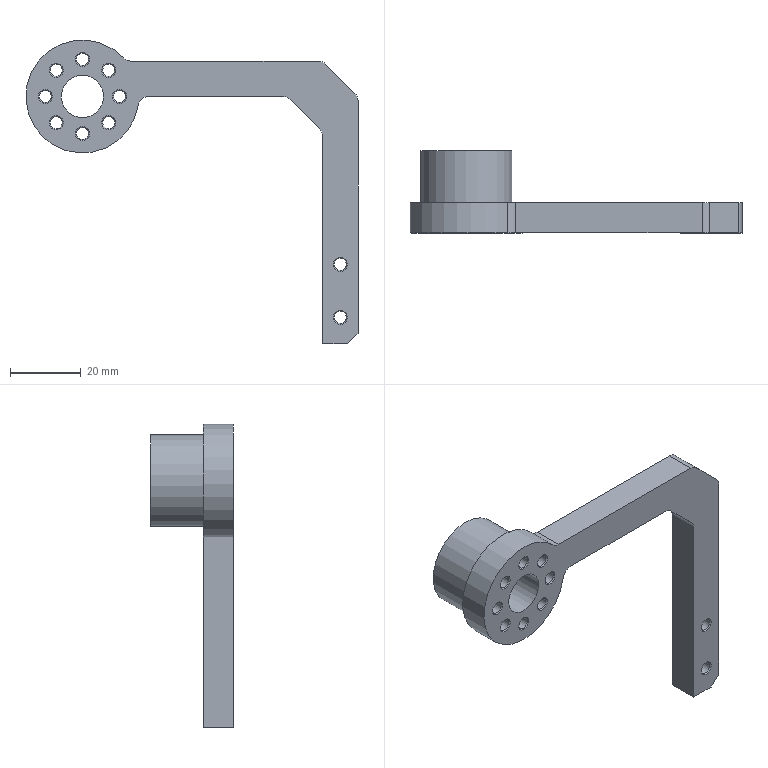Part | NX | features DATUM_CSYS 12, SKETCH 11, SIMPLE HOLE 10, HOLE PACKAGE 9, EXTRACT_FACE 8, Instance Feature 7, CHAMFER 3, BLEND 2, CPROJ 1, EXTRUDE 1, OFFSET_REGION 1, Pattern Feature 1, SWP104 1 | 1 solid | 52 faces | box 93.991 x 23.3 x 85.991 mm | volume 20704 mm3 | cylinder 20 | cone 20 | plane 12 | commonest cylinder face diameters 3.4 x10 6 x6 11.954 x1 25.981 x1 29.983 x1 31.983 x1
STEP:
#1=CARTESIAN_POINT('',(0.,-23.4,-5.977));
#2=VERTEX_POINT('',#1);
#3=CARTESIAN_POINT('',(0.,-23.4,0.));
#4=DIRECTION('',(0.,-1.,0.));
#5=DIRECTION('',(0.,0.,-1.));
#6=AXIS2_PLACEMENT_3D('',#3,#4,#5);
#7=CIRCLE('',#6,5.977);
#8=EDGE_CURVE('',#2,#2,#7,.T.);
#9=ORIENTED_EDGE('',*,*,#8,.T.);
#10=EDGE_LOOP('',(#9));
#11=FACE_BOUND('',#10,.T.);
#12=CARTESIAN_POINT('',(0.,-0.1,-5.977));
#13=VERTEX_POINT('',#12);
#14=CARTESIAN_POINT('',(0.,-0.1,0.));
#15=DIRECTION('',(0.,-1.,0.));
#16=DIRECTION('',(0.,0.,-1.));
#17=AXIS2_PLACEMENT_3D('',#14,#15,#16);
#18=CIRCLE('',#17,5.977);
#19=EDGE_CURVE('',#13,#13,#18,.T.);
#20=ORIENTED_EDGE('',*,*,#19,.F.);
#21=EDGE_LOOP('',(#20));
#22=FACE_BOUND('',#21,.T.);
#23=CARTESIAN_POINT('',(0.,0.,0.));
#24=DIRECTION('',(0.,-1.,0.));
#25=DIRECTION('',(0.,0.,-1.));
#26=AXIS2_PLACEMENT_3D('',#23,#24,#25);
#27=CYLINDRICAL_SURFACE('',#26,5.977);
#28=ADVANCED_FACE('',(#11,#22),#27,.F.);
#29=CARTESIAN_POINT('',(73.,-23.4,-64.5));
#30=VERTEX_POINT('',#29);
#31=CARTESIAN_POINT('',(73.,-23.4,-62.5));
#32=DIRECTION('',(0.,-1.,0.));
#33=DIRECTION('',(0.,0.,-1.));
#34=AXIS2_PLACEMENT_3D('',#31,#32,#33);
#35=CIRCLE('',#34,2.);
#36=EDGE_CURVE('',#30,#30,#35,.F.);
#37=ORIENTED_EDGE('',*,*,#36,.T.);
#38=EDGE_LOOP('',(#37));
#39=FACE_BOUND('',#38,.T.);
#40=CARTESIAN_POINT('',(73.,-23.4,-49.5));
#41=VERTEX_POINT('',#40);
#42=CARTESIAN_POINT('',(73.,-23.4,-47.5));
#43=DIRECTION('',(0.,-1.,0.));
#44=DIRECTION('',(0.,0.,-1.));
#45=AXIS2_PLACEMENT_3D('',#42,#43,#44);
#46=CIRCLE('',#45,2.);
#47=EDGE_CURVE('',#41,#41,#46,.F.);
#48=ORIENTED_EDGE('',*,*,#47,.T.);
#49=EDGE_LOOP('',(#48));
#50=FACE_BOUND('',#49,.T.);
#51=CARTESIAN_POINT('',(7.425,-23.4,5.425));
#52=VERTEX_POINT('',#51);
#53=CARTESIAN_POINT('',(7.425,-23.4,7.425));
#54=DIRECTION('',(0.,-1.,0.));
#55=DIRECTION('',(0.,0.,-1.));
#56=AXIS2_PLACEMENT_3D('',#53,#54,#55);
#57=CIRCLE('',#56,2.);
#58=EDGE_CURVE('',#52,#52,#57,.F.);
#59=ORIENTED_EDGE('',*,*,#58,.T.);
#60=EDGE_LOOP('',(#59));
#61=FACE_BOUND('',#60,.T.);
#62=CARTESIAN_POINT('',(10.5,-23.4,-2.));
#63=VERTEX_POINT('',#62);
#64=CARTESIAN_POINT('',(10.5,-23.4,0.));
#65=DIRECTION('',(0.,-1.,0.));
#66=DIRECTION('',(0.,0.,-1.));
#67=AXIS2_PLACEMENT_3D('',#64,#65,#66);
#68=CIRCLE('',#67,2.);
#69=EDGE_CURVE('',#63,#63,#68,.F.);
#70=ORIENTED_EDGE('',*,*,#69,.T.);
#71=EDGE_LOOP('',(#70));
#72=FACE_BOUND('',#71,.T.);
#73=CARTESIAN_POINT('',(7.425,-23.4,-9.425));
#74=VERTEX_POINT('',#73);
#75=CARTESIAN_POINT('',(7.425,-23.4,-7.425));
#76=DIRECTION('',(0.,-1.,0.));
#77=DIRECTION('',(0.,0.,-1.));
#78=AXIS2_PLACEMENT_3D('',#75,#76,#77);
#79=CIRCLE('',#78,2.);
#80=EDGE_CURVE('',#74,#74,#79,.F.);
#81=ORIENTED_EDGE('',*,*,#80,.T.);
#82=EDGE_LOOP('',(#81));
#83=FACE_BOUND('',#82,.T.);
#84=CARTESIAN_POINT('',(0.,-23.4,-12.5));
#85=VERTEX_POINT('',#84);
#86=CARTESIAN_POINT('',(0.,-23.4,-10.5));
#87=DIRECTION('',(0.,-1.,0.));
#88=DIRECTION('',(0.,0.,-1.));
#89=AXIS2_PLACEMENT_3D('',#86,#87,#88);
#90=CIRCLE('',#89,2.);
#91=EDGE_CURVE('',#85,#85,#90,.F.);
#92=ORIENTED_EDGE('',*,*,#91,.T.);
#93=EDGE_LOOP('',(#92));
#94=FACE_BOUND('',#93,.T.);
#95=CARTESIAN_POINT('',(-7.425,-23.4,-9.425));
#96=VERTEX_POINT('',#95);
#97=CARTESIAN_POINT('',(-7.425,-23.4,-7.425));
#98=DIRECTION('',(0.,-1.,0.));
#99=DIRECTION('',(0.,0.,-1.));
#100=AXIS2_PLACEMENT_3D('',#97,#98,#99);
#101=CIRCLE('',#100,2.);
#102=EDGE_CURVE('',#96,#96,#101,.F.);
#103=ORIENTED_EDGE('',*,*,#102,.T.);
#104=EDGE_LOOP('',(#103));
#105=FACE_BOUND('',#104,.T.);
#106=CARTESIAN_POINT('',(-10.5,-23.4,-2.));
#107=VERTEX_POINT('',#106);
#108=CARTESIAN_POINT('',(-10.5,-23.4,0.));
#109=DIRECTION('',(0.,-1.,0.));
#110=DIRECTION('',(0.,0.,-1.));
#111=AXIS2_PLACEMENT_3D('',#108,#109,#110);
#112=CIRCLE('',#111,2.);
#113=EDGE_CURVE('',#107,#107,#112,.F.);
#114=ORIENTED_EDGE('',*,*,#113,.T.);
#115=EDGE_LOOP('',(#114));
#116=FACE_BOUND('',#115,.T.);
#117=CARTESIAN_POINT('',(-7.425,-23.4,5.425));
#118=VERTEX_POINT('',#117);
#119=CARTESIAN_POINT('',(-7.425,-23.4,7.425));
#120=DIRECTION('',(0.,-1.,0.));
#121=DIRECTION('',(0.,0.,-1.));
#122=AXIS2_PLACEMENT_3D('',#119,#120,#121);
#123=CIRCLE('',#122,2.);
#124=EDGE_CURVE('',#118,#118,#123,.F.);
#125=ORIENTED_EDGE('',*,*,#124,.T.);
#126=EDGE_LOOP('',(#125));
#127=FACE_BOUND('',#126,.T.);
#128=CARTESIAN_POINT('',(0.,-23.4,8.5));
#129=VERTEX_POINT('',#128);
#130=CARTESIAN_POINT('',(0.,-23.4,10.5));
#131=DIRECTION('',(0.,-1.,0.));
#132=DIRECTION('',(0.,0.,-1.));
#133=AXIS2_PLACEMENT_3D('',#130,#131,#132);
#134=CIRCLE('',#133,2.);
#135=EDGE_CURVE('',#129,#129,#134,.F.);
#136=ORIENTED_EDGE('',*,*,#135,.T.);
#137=EDGE_LOOP('',(#136));
#138=FACE_BOUND('',#137,.T.);
#139=CARTESIAN_POINT('',(68.,-23.4,-70.));
#140=VERTEX_POINT('',#139);
#141=CARTESIAN_POINT('',(75.,-23.4,-70.));
#142=VERTEX_POINT('',#141);
#143=CARTESIAN_POINT('',(68.,-23.4,-70.));
#144=DIRECTION('',(1.,0.,0.));
#145=VECTOR('',#144,1000.);
#146=LINE('',#143,#145);
#147=EDGE_CURVE('',#140,#142,#146,.T.);
#148=ORIENTED_EDGE('',*,*,#147,.T.);
#149=CARTESIAN_POINT('',(78.,-23.4,-67.));
#150=VERTEX_POINT('',#149);
#151=CARTESIAN_POINT('',(75.489,-23.4,-69.511));
#152=DIRECTION('',(-0.7071,0.,-0.7071));
#153=VECTOR('',#152,1000.);
#154=LINE('',#151,#153);
#155=EDGE_CURVE('',#142,#150,#154,.F.);
#156=ORIENTED_EDGE('',*,*,#155,.T.);
#157=CARTESIAN_POINT('',(78.,-23.4,-1.243));
#158=VERTEX_POINT('',#157);
#159=CARTESIAN_POINT('',(78.,-23.4,0.));
#160=DIRECTION('',(0.,0.,1.));
#161=VECTOR('',#160,1000.);
#162=LINE('',#159,#161);
#163=EDGE_CURVE('',#150,#158,#162,.T.);
#164=ORIENTED_EDGE('',*,*,#163,.T.);
#165=CARTESIAN_POINT('',(77.121,-23.4,0.8787));
#166=VERTEX_POINT('',#165);
#167=CARTESIAN_POINT('',(75.,-23.4,-1.243));
#168=DIRECTION('',(0.,-1.,0.));
#169=DIRECTION('',(0.,0.,-1.));
#170=AXIS2_PLACEMENT_3D('',#167,#168,#169);
#171=CIRCLE('',#170,3.);
#172=EDGE_CURVE('',#158,#166,#171,.T.);
#173=ORIENTED_EDGE('',*,*,#172,.T.);
#174=CARTESIAN_POINT('',(68.879,-23.4,9.121));
#175=VERTEX_POINT('',#174);
#176=CARTESIAN_POINT('',(41.989,-23.4,36.011));
#177=DIRECTION('',(0.7071,0.,-0.7071));
#178=VECTOR('',#177,1000.);
#179=LINE('',#176,#178);
#180=EDGE_CURVE('',#166,#175,#179,.F.);
#181=ORIENTED_EDGE('',*,*,#180,.T.);
#182=CARTESIAN_POINT('',(66.757,-23.4,10.));
#183=VERTEX_POINT('',#182);
#184=CARTESIAN_POINT('',(66.757,-23.4,7.));
#185=DIRECTION('',(0.,-1.,0.));
#186=DIRECTION('',(0.,0.,-1.));
#187=AXIS2_PLACEMENT_3D('',#184,#185,#186);
#188=CIRCLE('',#187,3.);
#189=EDGE_CURVE('',#175,#183,#188,.T.);
#190=ORIENTED_EDGE('',*,*,#189,.T.);
#191=CARTESIAN_POINT('',(13.845,-23.4,10.));
#192=VERTEX_POINT('',#191);
#193=CARTESIAN_POINT('',(68.,-23.4,10.));
#194=DIRECTION('',(-1.,0.,0.));
#195=VECTOR('',#194,1000.);
#196=LINE('',#193,#195);
#197=EDGE_CURVE('',#183,#192,#196,.T.);
#198=ORIENTED_EDGE('',*,*,#197,.T.);
#199=CARTESIAN_POINT('',(11.658,-23.4,10.946));
#200=VERTEX_POINT('',#199);
#201=CARTESIAN_POINT('',(13.845,-23.4,13.));
#202=DIRECTION('',(0.,-1.,0.));
#203=DIRECTION('',(0.,0.,-1.));
#204=AXIS2_PLACEMENT_3D('',#201,#202,#203);
#205=CIRCLE('',#204,3.);
#206=EDGE_CURVE('',#192,#200,#205,.F.);
#207=ORIENTED_EDGE('',*,*,#206,.T.);
#208=CARTESIAN_POINT('',(15.791,-23.4,-2.526));
#209=VERTEX_POINT('',#208);
#210=CARTESIAN_POINT('',(0.,-23.4,0.));
#211=DIRECTION('',(0.,-1.,0.));
#212=DIRECTION('',(0.,0.,-1.));
#213=AXIS2_PLACEMENT_3D('',#210,#211,#212);
#214=CIRCLE('',#213,15.991);
#215=EDGE_CURVE('',#200,#209,#214,.T.);
#216=ORIENTED_EDGE('',*,*,#215,.T.);
#217=CARTESIAN_POINT('',(18.753,-23.4,0.));
#218=VERTEX_POINT('',#217);
#219=CARTESIAN_POINT('',(18.753,-23.4,-3.));
#220=DIRECTION('',(0.,-1.,0.));
#221=DIRECTION('',(0.,0.,-1.));
#222=AXIS2_PLACEMENT_3D('',#219,#220,#221);
#223=CIRCLE('',#222,3.);
#224=EDGE_CURVE('',#209,#218,#223,.F.);
#225=ORIENTED_EDGE('',*,*,#224,.T.);
#226=CARTESIAN_POINT('',(56.757,-23.4,0.));
#227=VERTEX_POINT('',#226);
#228=CARTESIAN_POINT('',(15.991,-23.4,0.));
#229=DIRECTION('',(1.,0.,0.));
#230=VECTOR('',#229,1000.);
#231=LINE('',#228,#230);
#232=EDGE_CURVE('',#218,#227,#231,.T.);
#233=ORIENTED_EDGE('',*,*,#232,.T.);
#234=CARTESIAN_POINT('',(58.879,-23.4,-0.8787));
#235=VERTEX_POINT('',#234);
#236=CARTESIAN_POINT('',(56.757,-23.4,-3.));
#237=DIRECTION('',(0.,-1.,0.));
#238=DIRECTION('',(0.,0.,-1.));
#239=AXIS2_PLACEMENT_3D('',#236,#237,#238);
#240=CIRCLE('',#239,3.);
#241=EDGE_CURVE('',#227,#235,#240,.F.);
#242=ORIENTED_EDGE('',*,*,#241,.T.);
#243=CARTESIAN_POINT('',(67.121,-23.4,-9.121));
#244=VERTEX_POINT('',#243);
#245=CARTESIAN_POINT('',(58.,-23.4,0.));
#246=DIRECTION('',(-0.7071,0.,0.7071));
#247=VECTOR('',#246,1000.);
#248=LINE('',#245,#247);
#249=EDGE_CURVE('',#235,#244,#248,.F.);
#250=ORIENTED_EDGE('',*,*,#249,.T.);
#251=CARTESIAN_POINT('',(68.,-23.4,-11.243));
#252=VERTEX_POINT('',#251);
#253=CARTESIAN_POINT('',(65.,-23.4,-11.243));
#254=DIRECTION('',(0.,-1.,0.));
#255=DIRECTION('',(0.,0.,-1.));
#256=AXIS2_PLACEMENT_3D('',#253,#254,#255);
#257=CIRCLE('',#256,3.);
#258=EDGE_CURVE('',#244,#252,#257,.F.);
#259=ORIENTED_EDGE('',*,*,#258,.T.);
#260=CARTESIAN_POINT('',(68.,-23.4,0.));
#261=DIRECTION('',(0.,0.,-1.));
#262=VECTOR('',#261,1000.);
#263=LINE('',#260,#262);
#264=EDGE_CURVE('',#252,#140,#263,.T.);
#265=ORIENTED_EDGE('',*,*,#264,.T.);
#266=EDGE_LOOP('',(#148,#156,#164,#173,#181,#190,#198,#207,#216,#225,#233,#242,#250,#259,#265));
#267=FACE_BOUND('',#266,.T.);
#268=ORIENTED_EDGE('',*,*,#8,.F.);
#269=EDGE_LOOP('',(#268));
#270=FACE_BOUND('',#269,.T.);
#271=CARTESIAN_POINT('',(5.977,-23.4,0.));
#272=DIRECTION('',(0.,-1.,0.));
#273=DIRECTION('',(0.,0.,-1.));
#274=AXIS2_PLACEMENT_3D('',#271,#272,#273);
#275=PLANE('',#274);
#276=ADVANCED_FACE('',(#39,#50,#61,#72,#83,#94,#105,#116,#127,#138,#267,#270),#275,.T.);
#277=CARTESIAN_POINT('',(11.658,-14.9,10.946));
#278=VERTEX_POINT('',#277);
#279=CARTESIAN_POINT('',(15.791,-14.9,-2.526));
#280=VERTEX_POINT('',#279);
#281=CARTESIAN_POINT('',(0.,-14.9,0.));
#282=DIRECTION('',(0.,-1.,0.));
#283=DIRECTION('',(0.,0.,-1.));
#284=AXIS2_PLACEMENT_3D('',#281,#282,#283);
#285=CIRCLE('',#284,15.991);
#286=EDGE_CURVE('',#278,#280,#285,.T.);
#287=ORIENTED_EDGE('',*,*,#286,.T.);
#288=CARTESIAN_POINT('',(15.791,0.,-2.526));
#289=DIRECTION('',(0.,-1.,0.));
#290=VECTOR('',#289,1000.);
#291=LINE('',#288,#290);
#292=EDGE_CURVE('',#280,#209,#291,.T.);
#293=ORIENTED_EDGE('',*,*,#292,.T.);
#294=ORIENTED_EDGE('',*,*,#215,.F.);
#295=CARTESIAN_POINT('',(11.658,0.,10.946));
#296=DIRECTION('',(0.,-1.,0.));
#297=VECTOR('',#296,1000.);
#298=LINE('',#295,#297);
#299=EDGE_CURVE('',#200,#278,#298,.F.);
#300=ORIENTED_EDGE('',*,*,#299,.T.);
#301=EDGE_LOOP('',(#287,#293,#294,#300));
#302=FACE_BOUND('',#301,.T.);
#303=CARTESIAN_POINT('',(0.,0.,0.));
#304=DIRECTION('',(0.,-1.,0.));
#305=DIRECTION('',(0.,0.,-1.));
#306=AXIS2_PLACEMENT_3D('',#303,#304,#305);
#307=CYLINDRICAL_SURFACE('',#306,15.991);
#308=ADVANCED_FACE('',(#302),#307,.T.);
#309=CARTESIAN_POINT('',(73.,-14.9,-60.5));
#310=VERTEX_POINT('',#309);
#311=CARTESIAN_POINT('',(73.,-14.9,-62.5));
#312=DIRECTION('',(0.,1.,0.));
#313=DIRECTION('',(0.,0.,1.));
#314=AXIS2_PLACEMENT_3D('',#311,#312,#313);
#315=CIRCLE('',#314,2.);
#316=EDGE_CURVE('',#310,#310,#315,.F.);
#317=ORIENTED_EDGE('',*,*,#316,.T.);
#318=EDGE_LOOP('',(#317));
#319=FACE_BOUND('',#318,.T.);
#320=CARTESIAN_POINT('',(73.,-14.9,-45.5));
#321=VERTEX_POINT('',#320);
#322=CARTESIAN_POINT('',(73.,-14.9,-47.5));
#323=DIRECTION('',(0.,1.,0.));
#324=DIRECTION('',(0.,0.,1.));
#325=AXIS2_PLACEMENT_3D('',#322,#323,#324);
#326=CIRCLE('',#325,2.);
#327=EDGE_CURVE('',#321,#321,#326,.F.);
#328=ORIENTED_EDGE('',*,*,#327,.T.);
#329=EDGE_LOOP('',(#328));
#330=FACE_BOUND('',#329,.T.);
#331=CARTESIAN_POINT('',(0.,-14.9,-14.991));
#332=VERTEX_POINT('',#331);
#333=CARTESIAN_POINT('',(0.,-14.9,0.));
#334=DIRECTION('',(0.,-1.,0.));
#335=DIRECTION('',(0.,0.,-1.));
#336=AXIS2_PLACEMENT_3D('',#333,#334,#335);
#337=CIRCLE('',#336,14.991);
#338=EDGE_CURVE('',#332,#332,#337,.T.);
#339=ORIENTED_EDGE('',*,*,#338,.T.);
#340=EDGE_LOOP('',(#339));
#341=FACE_BOUND('',#340,.T.);
#342=CARTESIAN_POINT('',(78.,-14.9,-67.));
#343=VERTEX_POINT('',#342);
#344=CARTESIAN_POINT('',(78.,-14.9,-1.243));
#345=VERTEX_POINT('',#344);
#346=CARTESIAN_POINT('',(78.,-14.9,-70.));
#347=DIRECTION('',(0.,0.,1.));
#348=VECTOR('',#347,1000.);
#349=LINE('',#346,#348);
#350=EDGE_CURVE('',#343,#345,#349,.T.);
#351=ORIENTED_EDGE('',*,*,#350,.F.);
#352=CARTESIAN_POINT('',(75.,-14.9,-70.));
#353=VERTEX_POINT('',#352);
#354=CARTESIAN_POINT('',(80.496,-14.9,-64.504));
#355=DIRECTION('',(0.7071,0.,0.7071));
#356=VECTOR('',#355,1000.);
#357=LINE('',#354,#356);
#358=EDGE_CURVE('',#343,#353,#357,.F.);
#359=ORIENTED_EDGE('',*,*,#358,.T.);
#360=CARTESIAN_POINT('',(68.,-14.9,-70.));
#361=VERTEX_POINT('',#360);
#362=CARTESIAN_POINT('',(68.,-14.9,-70.));
#363=DIRECTION('',(1.,0.,0.));
#364=VECTOR('',#363,1000.);
#365=LINE('',#362,#364);
#366=EDGE_CURVE('',#361,#353,#365,.T.);
#367=ORIENTED_EDGE('',*,*,#366,.F.);
#368=CARTESIAN_POINT('',(68.,-14.9,-11.243));
#369=VERTEX_POINT('',#368);
#370=CARTESIAN_POINT('',(68.,-14.9,0.));
#371=DIRECTION('',(0.,0.,-1.));
#372=VECTOR('',#371,1000.);
#373=LINE('',#370,#372);
#374=EDGE_CURVE('',#369,#361,#373,.T.);
#375=ORIENTED_EDGE('',*,*,#374,.F.);
#376=CARTESIAN_POINT('',(67.121,-14.9,-9.121));
#377=VERTEX_POINT('',#376);
#378=CARTESIAN_POINT('',(65.,-14.9,-11.243));
#379=DIRECTION('',(0.,1.,0.));
#380=DIRECTION('',(0.,0.,1.));
#381=AXIS2_PLACEMENT_3D('',#378,#379,#380);
#382=CIRCLE('',#381,3.);
#383=EDGE_CURVE('',#369,#377,#382,.F.);
#384=ORIENTED_EDGE('',*,*,#383,.T.);
#385=CARTESIAN_POINT('',(58.879,-14.9,-0.8787));
#386=VERTEX_POINT('',#385);
#387=CARTESIAN_POINT('',(58.,-14.9,0.));
#388=DIRECTION('',(0.7071,0.,-0.7071));
#389=VECTOR('',#388,1000.);
#390=LINE('',#387,#389);
#391=EDGE_CURVE('',#377,#386,#390,.F.);
#392=ORIENTED_EDGE('',*,*,#391,.T.);
#393=CARTESIAN_POINT('',(56.757,-14.9,0.));
#394=VERTEX_POINT('',#393);
#395=CARTESIAN_POINT('',(56.757,-14.9,-3.));
#396=DIRECTION('',(0.,1.,0.));
#397=DIRECTION('',(0.,0.,1.));
#398=AXIS2_PLACEMENT_3D('',#395,#396,#397);
#399=CIRCLE('',#398,3.);
#400=EDGE_CURVE('',#386,#394,#399,.F.);
#401=ORIENTED_EDGE('',*,*,#400,.T.);
#402=CARTESIAN_POINT('',(18.753,-14.9,0.));
#403=VERTEX_POINT('',#402);
#404=CARTESIAN_POINT('',(15.991,-14.9,0.));
#405=DIRECTION('',(1.,0.,0.));
#406=VECTOR('',#405,1000.);
#407=LINE('',#404,#406);
#408=EDGE_CURVE('',#403,#394,#407,.T.);
#409=ORIENTED_EDGE('',*,*,#408,.F.);
#410=CARTESIAN_POINT('',(18.753,-14.9,-3.));
#411=DIRECTION('',(0.,1.,0.));
#412=DIRECTION('',(0.,0.,1.));
#413=AXIS2_PLACEMENT_3D('',#410,#411,#412);
#414=CIRCLE('',#413,3.);
#415=EDGE_CURVE('',#403,#280,#414,.F.);
#416=ORIENTED_EDGE('',*,*,#415,.T.);
#417=ORIENTED_EDGE('',*,*,#286,.F.);
#418=CARTESIAN_POINT('',(13.845,-14.9,10.));
#419=VERTEX_POINT('',#418);
#420=CARTESIAN_POINT('',(13.845,-14.9,13.));
#421=DIRECTION('',(0.,1.,0.));
#422=DIRECTION('',(0.,0.,1.));
#423=AXIS2_PLACEMENT_3D('',#420,#421,#422);
#424=CIRCLE('',#423,3.);
#425=EDGE_CURVE('',#278,#419,#424,.F.);
#426=ORIENTED_EDGE('',*,*,#425,.T.);
#427=CARTESIAN_POINT('',(66.757,-14.9,10.));
#428=VERTEX_POINT('',#427);
#429=CARTESIAN_POINT('',(78.,-14.9,10.));
#430=DIRECTION('',(-1.,0.,0.));
#431=VECTOR('',#430,1000.);
#432=LINE('',#429,#431);
#433=EDGE_CURVE('',#428,#419,#432,.T.);
#434=ORIENTED_EDGE('',*,*,#433,.F.);
#435=CARTESIAN_POINT('',(68.879,-14.9,9.121));
#436=VERTEX_POINT('',#435);
#437=CARTESIAN_POINT('',(66.757,-14.9,7.));
#438=DIRECTION('',(0.,1.,0.));
#439=DIRECTION('',(0.,0.,1.));
#440=AXIS2_PLACEMENT_3D('',#437,#438,#439);
#441=CIRCLE('',#440,3.);
#442=EDGE_CURVE('',#428,#436,#441,.T.);
#443=ORIENTED_EDGE('',*,*,#442,.T.);
#444=CARTESIAN_POINT('',(77.121,-14.9,0.8787));
#445=VERTEX_POINT('',#444);
#446=CARTESIAN_POINT('',(46.996,-14.9,31.004));
#447=DIRECTION('',(-0.7071,0.,0.7071));
#448=VECTOR('',#447,1000.);
#449=LINE('',#446,#448);
#450=EDGE_CURVE('',#436,#445,#449,.F.);
#451=ORIENTED_EDGE('',*,*,#450,.T.);
#452=CARTESIAN_POINT('',(75.,-14.9,-1.243));
#453=DIRECTION('',(0.,1.,0.));
#454=DIRECTION('',(0.,0.,1.));
#455=AXIS2_PLACEMENT_3D('',#452,#453,#454);
#456=CIRCLE('',#455,3.);
#457=EDGE_CURVE('',#445,#345,#456,.T.);
#458=ORIENTED_EDGE('',*,*,#457,.T.);
#459=EDGE_LOOP('',(#351,#359,#367,#375,#384,#392,#401,#409,#416,#417,#426,#434,#443,#451,#458));
#460=FACE_BOUND('',#459,.T.);
#461=CARTESIAN_POINT('',(15.991,-14.9,0.));
#462=DIRECTION('',(0.,1.,0.));
#463=DIRECTION('',(0.,0.,1.));
#464=AXIS2_PLACEMENT_3D('',#461,#462,#463);
#465=PLANE('',#464);
#466=ADVANCED_FACE('',(#319,#330,#341,#460),#465,.T.);
#467=CARTESIAN_POINT('',(0.,-19.4,14.991));
#468=VERTEX_POINT('',#467);
#469=CARTESIAN_POINT('',(0.,-19.4,0.));
#470=DIRECTION('',(0.,1.,0.));
#471=DIRECTION('',(0.,0.,1.));
#472=AXIS2_PLACEMENT_3D('',#469,#470,#471);
#473=CIRCLE('',#472,14.991);
#474=EDGE_CURVE('',#468,#468,#473,.F.);
#475=ORIENTED_EDGE('',*,*,#474,.T.);
#476=EDGE_LOOP('',(#475));
#477=FACE_BOUND('',#476,.T.);
#478=ORIENTED_EDGE('',*,*,#338,.F.);
#479=EDGE_LOOP('',(#478));
#480=FACE_BOUND('',#479,.T.);
#481=CARTESIAN_POINT('',(0.,0.,0.));
#482=DIRECTION('',(0.,-1.,0.));
#483=DIRECTION('',(0.,0.,-1.));
#484=AXIS2_PLACEMENT_3D('',#481,#482,#483);
#485=CYLINDRICAL_SURFACE('',#484,14.991);
#486=ADVANCED_FACE('',(#477,#480),#485,.F.);
#487=CARTESIAN_POINT('',(0.,-19.4,12.991));
#488=VERTEX_POINT('',#487);
#489=CARTESIAN_POINT('',(0.,-19.4,0.));
#490=DIRECTION('',(0.,1.,0.));
#491=DIRECTION('',(0.,0.,1.));
#492=AXIS2_PLACEMENT_3D('',#489,#490,#491);
#493=CIRCLE('',#492,12.991);
#494=EDGE_CURVE('',#488,#488,#493,.F.);
#495=ORIENTED_EDGE('',*,*,#494,.T.);
#496=EDGE_LOOP('',(#495));
#497=FACE_BOUND('',#496,.T.);
#498=ORIENTED_EDGE('',*,*,#474,.F.);
#499=EDGE_LOOP('',(#498));
#500=FACE_BOUND('',#499,.T.);
#501=CARTESIAN_POINT('',(14.991,-19.4,0.));
#502=DIRECTION('',(0.,1.,0.));
#503=DIRECTION('',(0.,0.,1.));
#504=AXIS2_PLACEMENT_3D('',#501,#502,#503);
#505=PLANE('',#504);
#506=ADVANCED_FACE('',(#497,#500),#505,.T.);
#507=CARTESIAN_POINT('',(0.,-0.1,-12.991));
#508=VERTEX_POINT('',#507);
#509=CARTESIAN_POINT('',(0.,-0.1,0.));
#510=DIRECTION('',(0.,-1.,0.));
#511=DIRECTION('',(0.,0.,-1.));
#512=AXIS2_PLACEMENT_3D('',#509,#510,#511);
#513=CIRCLE('',#512,12.991);
#514=EDGE_CURVE('',#508,#508,#513,.T.);
#515=ORIENTED_EDGE('',*,*,#514,.T.);
#516=EDGE_LOOP('',(#515));
#517=FACE_BOUND('',#516,.T.);
#518=ORIENTED_EDGE('',*,*,#494,.F.);
#519=EDGE_LOOP('',(#518));
#520=FACE_BOUND('',#519,.T.);
#521=CARTESIAN_POINT('',(0.,0.,0.));
#522=DIRECTION('',(0.,-1.,0.));
#523=DIRECTION('',(0.,0.,-1.));
#524=AXIS2_PLACEMENT_3D('',#521,#522,#523);
#525=CYLINDRICAL_SURFACE('',#524,12.991);
#526=ADVANCED_FACE('',(#517,#520),#525,.T.);
#527=CARTESIAN_POINT('',(7.425,-0.1,9.425));
#528=VERTEX_POINT('',#527);
#529=CARTESIAN_POINT('',(7.425,-0.1,7.425));
#530=DIRECTION('',(0.,1.,0.));
#531=DIRECTION('',(0.,0.,1.));
#532=AXIS2_PLACEMENT_3D('',#529,#530,#531);
#533=CIRCLE('',#532,2.);
#534=EDGE_CURVE('',#528,#528,#533,.F.);
#535=ORIENTED_EDGE('',*,*,#534,.T.);
#536=EDGE_LOOP('',(#535));
#537=FACE_BOUND('',#536,.T.);
#538=CARTESIAN_POINT('',(10.5,-0.1,2.));
#539=VERTEX_POINT('',#538);
#540=CARTESIAN_POINT('',(10.5,-0.1,0.));
#541=DIRECTION('',(0.,1.,0.));
#542=DIRECTION('',(0.,0.,1.));
#543=AXIS2_PLACEMENT_3D('',#540,#541,#542);
#544=CIRCLE('',#543,2.);
#545=EDGE_CURVE('',#539,#539,#544,.F.);
#546=ORIENTED_EDGE('',*,*,#545,.T.);
#547=EDGE_LOOP('',(#546));
#548=FACE_BOUND('',#547,.T.);
#549=CARTESIAN_POINT('',(7.425,-0.1,-5.425));
#550=VERTEX_POINT('',#549);
#551=CARTESIAN_POINT('',(7.425,-0.1,-7.425));
#552=DIRECTION('',(0.,1.,0.));
#553=DIRECTION('',(0.,0.,1.));
#554=AXIS2_PLACEMENT_3D('',#551,#552,#553);
#555=CIRCLE('',#554,2.);
#556=EDGE_CURVE('',#550,#550,#555,.F.);
#557=ORIENTED_EDGE('',*,*,#556,.T.);
#558=EDGE_LOOP('',(#557));
#559=FACE_BOUND('',#558,.T.);
#560=CARTESIAN_POINT('',(0.,-0.1,-8.5));
#561=VERTEX_POINT('',#560);
#562=CARTESIAN_POINT('',(0.,-0.1,-10.5));
#563=DIRECTION('',(0.,1.,0.));
#564=DIRECTION('',(0.,0.,1.));
#565=AXIS2_PLACEMENT_3D('',#562,#563,#564);
#566=CIRCLE('',#565,2.);
#567=EDGE_CURVE('',#561,#561,#566,.F.);
#568=ORIENTED_EDGE('',*,*,#567,.T.);
#569=EDGE_LOOP('',(#568));
#570=FACE_BOUND('',#569,.T.);
#571=CARTESIAN_POINT('',(-7.425,-0.1,-5.425));
#572=VERTEX_POINT('',#571);
#573=CARTESIAN_POINT('',(-7.425,-0.1,-7.425));
#574=DIRECTION('',(0.,1.,0.));
#575=DIRECTION('',(0.,0.,1.));
#576=AXIS2_PLACEMENT_3D('',#573,#574,#575);
#577=CIRCLE('',#576,2.);
#578=EDGE_CURVE('',#572,#572,#577,.F.);
#579=ORIENTED_EDGE('',*,*,#578,.T.);
#580=EDGE_LOOP('',(#579));
#581=FACE_BOUND('',#580,.T.);
#582=CARTESIAN_POINT('',(-10.5,-0.1,2.));
#583=VERTEX_POINT('',#582);
#584=CARTESIAN_POINT('',(-10.5,-0.1,0.));
#585=DIRECTION('',(0.,1.,0.));
#586=DIRECTION('',(0.,0.,1.));
#587=AXIS2_PLACEMENT_3D('',#584,#585,#586);
#588=CIRCLE('',#587,2.);
#589=EDGE_CURVE('',#583,#583,#588,.F.);
#590=ORIENTED_EDGE('',*,*,#589,.T.);
#591=EDGE_LOOP('',(#590));
#592=FACE_BOUND('',#591,.T.);
#593=CARTESIAN_POINT('',(-7.425,-0.1,9.425));
#594=VERTEX_POINT('',#593);
#595=CARTESIAN_POINT('',(-7.425,-0.1,7.425));
#596=DIRECTION('',(0.,1.,0.));
#597=DIRECTION('',(0.,0.,1.));
#598=AXIS2_PLACEMENT_3D('',#595,#596,#597);
#599=CIRCLE('',#598,2.);
#600=EDGE_CURVE('',#594,#594,#599,.F.);
#601=ORIENTED_EDGE('',*,*,#600,.T.);
#602=EDGE_LOOP('',(#601));
#603=FACE_BOUND('',#602,.T.);
#604=CARTESIAN_POINT('',(0.,-0.1,12.5));
#605=VERTEX_POINT('',#604);
#606=CARTESIAN_POINT('',(0.,-0.1,10.5));
#607=DIRECTION('',(0.,1.,0.));
#608=DIRECTION('',(0.,0.,1.));
#609=AXIS2_PLACEMENT_3D('',#606,#607,#608);
#610=CIRCLE('',#609,2.);
#611=EDGE_CURVE('',#605,#605,#610,.F.);
#612=ORIENTED_EDGE('',*,*,#611,.T.);
#613=EDGE_LOOP('',(#612));
#614=FACE_BOUND('',#613,.T.);
#615=ORIENTED_EDGE('',*,*,#19,.T.);
#616=EDGE_LOOP('',(#615));
#617=FACE_BOUND('',#616,.T.);
#618=ORIENTED_EDGE('',*,*,#514,.F.);
#619=EDGE_LOOP('',(#618));
#620=FACE_BOUND('',#619,.T.);
#621=CARTESIAN_POINT('',(12.991,-0.1,0.));
#622=DIRECTION('',(0.,1.,0.));
#623=DIRECTION('',(0.,0.,1.));
#624=AXIS2_PLACEMENT_3D('',#621,#622,#623);
#625=PLANE('',#624);
#626=ADVANCED_FACE('',(#537,#548,#559,#570,#581,#592,#603,#614,#617,#620),#625,.T.);
#627=ORIENTED_EDGE('',*,*,#232,.F.);
#628=CARTESIAN_POINT('',(18.753,-14.9,0.));
#629=DIRECTION('',(0.,1.,0.));
#630=VECTOR('',#629,1000.);
#631=LINE('',#628,#630);
#632=EDGE_CURVE('',#218,#403,#631,.T.);
#633=ORIENTED_EDGE('',*,*,#632,.T.);
#634=ORIENTED_EDGE('',*,*,#408,.T.);
#635=CARTESIAN_POINT('',(56.757,-14.9,0.));
#636=DIRECTION('',(0.,1.,0.));
#637=VECTOR('',#636,1000.);
#638=LINE('',#635,#637);
#639=EDGE_CURVE('',#394,#227,#638,.F.);
#640=ORIENTED_EDGE('',*,*,#639,.T.);
#641=EDGE_LOOP('',(#627,#633,#634,#640));
#642=FACE_BOUND('',#641,.T.);
#643=CARTESIAN_POINT('',(15.991,-14.9,0.));
#644=DIRECTION('',(0.,0.,-1.));
#645=DIRECTION('',(-1.,0.,0.));
#646=AXIS2_PLACEMENT_3D('',#643,#644,#645);
#647=PLANE('',#646);
#648=ADVANCED_FACE('',(#642),#647,.T.);
#649=ORIENTED_EDGE('',*,*,#264,.F.);
#650=CARTESIAN_POINT('',(68.,-14.9,-11.243));
#651=DIRECTION('',(0.,-1.,0.));
#652=VECTOR('',#651,1000.);
#653=LINE('',#650,#652);
#654=EDGE_CURVE('',#252,#369,#653,.F.);
#655=ORIENTED_EDGE('',*,*,#654,.T.);
#656=ORIENTED_EDGE('',*,*,#374,.T.);
#657=CARTESIAN_POINT('',(68.,-14.9,-70.));
#658=DIRECTION('',(0.,-1.,0.));
#659=VECTOR('',#658,1000.);
#660=LINE('',#657,#659);
#661=EDGE_CURVE('',#361,#140,#660,.T.);
#662=ORIENTED_EDGE('',*,*,#661,.T.);
#663=EDGE_LOOP('',(#649,#655,#656,#662));
#664=FACE_BOUND('',#663,.T.);
#665=CARTESIAN_POINT('',(68.,-14.9,0.));
#666=DIRECTION('',(-1.,0.,0.));
#667=DIRECTION('',(0.,0.,1.));
#668=AXIS2_PLACEMENT_3D('',#665,#666,#667);
#669=PLANE('',#668);
#670=ADVANCED_FACE('',(#664),#669,.T.);
#671=ORIENTED_EDGE('',*,*,#366,.T.);
#672=CARTESIAN_POINT('',(75.,-14.9,-70.));
#673=DIRECTION('',(0.,-1.,0.));
#674=VECTOR('',#673,1000.);
#675=LINE('',#672,#674);
#676=EDGE_CURVE('',#353,#142,#675,.T.);
#677=ORIENTED_EDGE('',*,*,#676,.T.);
#678=ORIENTED_EDGE('',*,*,#147,.F.);
#679=ORIENTED_EDGE('',*,*,#661,.F.);
#680=EDGE_LOOP('',(#671,#677,#678,#679));
#681=FACE_BOUND('',#680,.T.);
#682=CARTESIAN_POINT('',(68.,-14.9,-70.));
#683=DIRECTION('',(0.,0.,-1.));
#684=DIRECTION('',(-1.,0.,0.));
#685=AXIS2_PLACEMENT_3D('',#682,#683,#684);
#686=PLANE('',#685);
#687=ADVANCED_FACE('',(#681),#686,.T.);
#688=ORIENTED_EDGE('',*,*,#163,.F.);
#689=CARTESIAN_POINT('',(78.,-14.9,-67.));
#690=DIRECTION('',(0.,1.,0.));
#691=VECTOR('',#690,1000.);
#692=LINE('',#689,#691);
#693=EDGE_CURVE('',#150,#343,#692,.T.);
#694=ORIENTED_EDGE('',*,*,#693,.T.);
#695=ORIENTED_EDGE('',*,*,#350,.T.);
#696=CARTESIAN_POINT('',(78.,-14.9,-1.243));
#697=DIRECTION('',(0.,1.,0.));
#698=VECTOR('',#697,1000.);
#699=LINE('',#696,#698);
#700=EDGE_CURVE('',#345,#158,#699,.F.);
#701=ORIENTED_EDGE('',*,*,#700,.T.);
#702=EDGE_LOOP('',(#688,#694,#695,#701));
#703=FACE_BOUND('',#702,.T.);
#704=CARTESIAN_POINT('',(78.,-14.9,0.));
#705=DIRECTION('',(1.,0.,0.));
#706=DIRECTION('',(0.,0.,-1.));
#707=AXIS2_PLACEMENT_3D('',#704,#705,#706);
#708=PLANE('',#707);
#709=ADVANCED_FACE('',(#703),#708,.T.);
#710=ORIENTED_EDGE('',*,*,#433,.T.);
#711=CARTESIAN_POINT('',(13.845,-23.4,10.));
#712=DIRECTION('',(0.,1.,0.));
#713=VECTOR('',#712,1000.);
#714=LINE('',#711,#713);
#715=EDGE_CURVE('',#419,#192,#714,.F.);
#716=ORIENTED_EDGE('',*,*,#715,.T.);
#717=ORIENTED_EDGE('',*,*,#197,.F.);
#718=CARTESIAN_POINT('',(66.757,-14.9,10.));
#719=DIRECTION('',(0.,-1.,0.));
#720=VECTOR('',#719,1000.);
#721=LINE('',#718,#720);
#722=EDGE_CURVE('',#183,#428,#721,.F.);
#723=ORIENTED_EDGE('',*,*,#722,.T.);
#724=EDGE_LOOP('',(#710,#716,#717,#723));
#725=FACE_BOUND('',#724,.T.);
#726=CARTESIAN_POINT('',(68.,-14.9,10.));
#727=DIRECTION('',(0.,0.,1.));
#728=DIRECTION('',(1.,0.,0.));
#729=AXIS2_PLACEMENT_3D('',#726,#727,#728);
#730=PLANE('',#729);
#731=ADVANCED_FACE('',(#725),#730,.T.);
#732=ORIENTED_EDGE('',*,*,#391,.F.);
#733=CARTESIAN_POINT('',(67.121,-14.9,-9.121));
#734=DIRECTION('',(0.,1.,0.));
#735=VECTOR('',#734,1000.);
#736=LINE('',#733,#735);
#737=EDGE_CURVE('',#377,#244,#736,.F.);
#738=ORIENTED_EDGE('',*,*,#737,.T.);
#739=ORIENTED_EDGE('',*,*,#249,.F.);
#740=CARTESIAN_POINT('',(58.879,-14.9,-0.8787));
#741=DIRECTION('',(0.,-1.,0.));
#742=VECTOR('',#741,1000.);
#743=LINE('',#740,#742);
#744=EDGE_CURVE('',#235,#386,#743,.F.);
#745=ORIENTED_EDGE('',*,*,#744,.T.);
#746=EDGE_LOOP('',(#732,#738,#739,#745));
#747=FACE_BOUND('',#746,.T.);
#748=CARTESIAN_POINT('',(58.,-14.9,0.));
#749=DIRECTION('',(-0.7071,0.,-0.7071));
#750=DIRECTION('',(0.,1.,0.));
#751=AXIS2_PLACEMENT_3D('',#748,#749,#750);
#752=PLANE('',#751);
#753=ADVANCED_FACE('',(#747),#752,.T.);
#754=ORIENTED_EDGE('',*,*,#180,.F.);
#755=CARTESIAN_POINT('',(77.121,-14.9,0.8787));
#756=DIRECTION('',(0.,-1.,0.));
#757=VECTOR('',#756,1000.);
#758=LINE('',#755,#757);
#759=EDGE_CURVE('',#166,#445,#758,.F.);
#760=ORIENTED_EDGE('',*,*,#759,.T.);
#761=ORIENTED_EDGE('',*,*,#450,.F.);
#762=CARTESIAN_POINT('',(68.879,-14.9,9.121));
#763=DIRECTION('',(0.,1.,0.));
#764=VECTOR('',#763,1000.);
#765=LINE('',#762,#764);
#766=EDGE_CURVE('',#436,#175,#765,.F.);
#767=ORIENTED_EDGE('',*,*,#766,.T.);
#768=EDGE_LOOP('',(#754,#760,#761,#767));
#769=FACE_BOUND('',#768,.T.);
#770=CARTESIAN_POINT('',(78.,-14.9,0.));
#771=DIRECTION('',(-0.7071,0.,-0.7071));
#772=DIRECTION('',(0.,-1.,0.));
#773=AXIS2_PLACEMENT_3D('',#770,#771,#772);
#774=PLANE('',#773);
#775=ADVANCED_FACE('',(#769),#774,.F.);
#776=ORIENTED_EDGE('',*,*,#258,.F.);
#777=ORIENTED_EDGE('',*,*,#737,.F.);
#778=ORIENTED_EDGE('',*,*,#383,.F.);
#779=ORIENTED_EDGE('',*,*,#654,.F.);
#780=EDGE_LOOP('',(#776,#777,#778,#779));
#781=FACE_BOUND('',#780,.T.);
#782=CARTESIAN_POINT('',(65.,-14.9,-11.243));
#783=DIRECTION('',(0.,-1.,0.));
#784=DIRECTION('',(0.,0.,-1.));
#785=AXIS2_PLACEMENT_3D('',#782,#783,#784);
#786=CYLINDRICAL_SURFACE('',#785,3.);
#787=ADVANCED_FACE('',(#781),#786,.F.);
#788=ORIENTED_EDGE('',*,*,#400,.F.);
#789=ORIENTED_EDGE('',*,*,#744,.F.);
#790=ORIENTED_EDGE('',*,*,#241,.F.);
#791=ORIENTED_EDGE('',*,*,#639,.F.);
#792=EDGE_LOOP('',(#788,#789,#790,#791));
#793=FACE_BOUND('',#792,.T.);
#794=CARTESIAN_POINT('',(56.757,-14.9,-3.));
#795=DIRECTION('',(0.,1.,0.));
#796=DIRECTION('',(0.,0.,1.));
#797=AXIS2_PLACEMENT_3D('',#794,#795,#796);
#798=CYLINDRICAL_SURFACE('',#797,3.);
#799=ADVANCED_FACE('',(#793),#798,.F.);
#800=ORIENTED_EDGE('',*,*,#457,.F.);
#801=ORIENTED_EDGE('',*,*,#759,.F.);
#802=ORIENTED_EDGE('',*,*,#172,.F.);
#803=ORIENTED_EDGE('',*,*,#700,.F.);
#804=EDGE_LOOP('',(#800,#801,#802,#803));
#805=FACE_BOUND('',#804,.T.);
#806=CARTESIAN_POINT('',(75.,-14.9,-1.243));
#807=DIRECTION('',(0.,1.,0.));
#808=DIRECTION('',(0.,0.,1.));
#809=AXIS2_PLACEMENT_3D('',#806,#807,#808);
#810=CYLINDRICAL_SURFACE('',#809,3.);
#811=ADVANCED_FACE('',(#805),#810,.T.);
#812=ORIENTED_EDGE('',*,*,#189,.F.);
#813=ORIENTED_EDGE('',*,*,#766,.F.);
#814=ORIENTED_EDGE('',*,*,#442,.F.);
#815=ORIENTED_EDGE('',*,*,#722,.F.);
#816=EDGE_LOOP('',(#812,#813,#814,#815));
#817=FACE_BOUND('',#816,.T.);
#818=CARTESIAN_POINT('',(66.757,-14.9,7.));
#819=DIRECTION('',(0.,-1.,0.));
#820=DIRECTION('',(0.,0.,-1.));
#821=AXIS2_PLACEMENT_3D('',#818,#819,#820);
#822=CYLINDRICAL_SURFACE('',#821,3.);
#823=ADVANCED_FACE('',(#817),#822,.T.);
#824=ORIENTED_EDGE('',*,*,#415,.F.);
#825=ORIENTED_EDGE('',*,*,#632,.F.);
#826=ORIENTED_EDGE('',*,*,#224,.F.);
#827=ORIENTED_EDGE('',*,*,#292,.F.);
#828=EDGE_LOOP('',(#824,#825,#826,#827));
#829=FACE_BOUND('',#828,.T.);
#830=CARTESIAN_POINT('',(18.753,0.,-3.));
#831=DIRECTION('',(0.,-1.,0.));
#832=DIRECTION('',(0.,0.,-1.));
#833=AXIS2_PLACEMENT_3D('',#830,#831,#832);
#834=CYLINDRICAL_SURFACE('',#833,3.);
#835=ADVANCED_FACE('',(#829),#834,.F.);
#836=ORIENTED_EDGE('',*,*,#425,.F.);
#837=ORIENTED_EDGE('',*,*,#299,.F.);
#838=ORIENTED_EDGE('',*,*,#206,.F.);
#839=ORIENTED_EDGE('',*,*,#715,.F.);
#840=EDGE_LOOP('',(#836,#837,#838,#839));
#841=FACE_BOUND('',#840,.T.);
#842=CARTESIAN_POINT('',(13.845,0.,13.));
#843=DIRECTION('',(0.,-1.,0.));
#844=DIRECTION('',(0.,0.,-1.));
#845=AXIS2_PLACEMENT_3D('',#842,#843,#844);
#846=CYLINDRICAL_SURFACE('',#845,3.);
#847=ADVANCED_FACE('',(#841),#846,.F.);
#848=ORIENTED_EDGE('',*,*,#358,.F.);
#849=ORIENTED_EDGE('',*,*,#693,.F.);
#850=ORIENTED_EDGE('',*,*,#155,.F.);
#851=ORIENTED_EDGE('',*,*,#676,.F.);
#852=EDGE_LOOP('',(#848,#849,#850,#851));
#853=FACE_BOUND('',#852,.T.);
#854=CARTESIAN_POINT('',(75.,-14.9,-70.));
#855=DIRECTION('',(-0.7071,0.,0.7071));
#856=DIRECTION('',(0.,-1.,0.));
#857=AXIS2_PLACEMENT_3D('',#854,#855,#856);
#858=PLANE('',#857);
#859=ADVANCED_FACE('',(#853),#858,.F.);
#860=CARTESIAN_POINT('',(0.,-0.4,12.2));
#861=VERTEX_POINT('',#860);
#862=CARTESIAN_POINT('',(0.,-0.4,10.5));
#863=DIRECTION('',(0.,1.,0.));
#864=DIRECTION('',(0.,0.,1.));
#865=AXIS2_PLACEMENT_3D('',#862,#863,#864);
#866=CIRCLE('',#865,1.7);
#867=EDGE_CURVE('',#861,#861,#866,.T.);
#868=ORIENTED_EDGE('',*,*,#867,.T.);
#869=EDGE_LOOP('',(#868));
#870=FACE_BOUND('',#869,.T.);
#871=CARTESIAN_POINT('',(0.,-23.1,8.8));
#872=VERTEX_POINT('',#871);
#873=CARTESIAN_POINT('',(0.,-23.1,10.5));
#874=DIRECTION('',(0.,-1.,0.));
#875=DIRECTION('',(0.,0.,-1.));
#876=AXIS2_PLACEMENT_3D('',#873,#874,#875);
#877=CIRCLE('',#876,1.7);
#878=EDGE_CURVE('',#872,#872,#877,.T.);
#879=ORIENTED_EDGE('',*,*,#878,.T.);
#880=EDGE_LOOP('',(#879));
#881=FACE_BOUND('',#880,.T.);
#882=CARTESIAN_POINT('',(0.,-23.4,10.5));
#883=DIRECTION('',(0.,1.,0.));
#884=DIRECTION('',(0.,0.,1.));
#885=AXIS2_PLACEMENT_3D('',#882,#883,#884);
#886=CYLINDRICAL_SURFACE('',#885,1.7);
#887=ADVANCED_FACE('',(#870,#881),#886,.F.);
#888=ORIENTED_EDGE('',*,*,#878,.F.);
#889=EDGE_LOOP('',(#888));
#890=FACE_BOUND('',#889,.T.);
#891=ORIENTED_EDGE('',*,*,#135,.F.);
#892=EDGE_LOOP('',(#891));
#893=FACE_BOUND('',#892,.T.);
#894=CARTESIAN_POINT('',(0.,-23.4,10.5));
#895=DIRECTION('',(0.,-1.,0.));
#896=DIRECTION('',(0.,0.,-1.));
#897=AXIS2_PLACEMENT_3D('',#894,#895,#896);
#898=CONICAL_SURFACE('',#897,2.,0.7854);
#899=ADVANCED_FACE('',(#890,#893),#898,.F.);
#900=ORIENTED_EDGE('',*,*,#611,.F.);
#901=EDGE_LOOP('',(#900));
#902=FACE_BOUND('',#901,.T.);
#903=ORIENTED_EDGE('',*,*,#867,.F.);
#904=EDGE_LOOP('',(#903));
#905=FACE_BOUND('',#904,.T.);
#906=CARTESIAN_POINT('',(0.,-0.4,10.5));
#907=DIRECTION('',(0.,1.,0.));
#908=DIRECTION('',(0.,0.,1.));
#909=AXIS2_PLACEMENT_3D('',#906,#907,#908);
#910=CONICAL_SURFACE('',#909,1.7,0.7854);
#911=ADVANCED_FACE('',(#902,#905),#910,.F.);
#912=CARTESIAN_POINT('',(-7.425,-0.4,9.125));
#913=VERTEX_POINT('',#912);
#914=CARTESIAN_POINT('',(-7.425,-0.4,7.425));
#915=DIRECTION('',(0.,1.,0.));
#916=DIRECTION('',(0.,0.,1.));
#917=AXIS2_PLACEMENT_3D('',#914,#915,#916);
#918=CIRCLE('',#917,1.7);
#919=EDGE_CURVE('',#913,#913,#918,.T.);
#920=ORIENTED_EDGE('',*,*,#919,.T.);
#921=EDGE_LOOP('',(#920));
#922=FACE_BOUND('',#921,.T.);
#923=CARTESIAN_POINT('',(-7.425,-23.1,5.725));
#924=VERTEX_POINT('',#923);
#925=CARTESIAN_POINT('',(-7.425,-23.1,7.425));
#926=DIRECTION('',(0.,-1.,0.));
#927=DIRECTION('',(0.,0.,-1.));
#928=AXIS2_PLACEMENT_3D('',#925,#926,#927);
#929=CIRCLE('',#928,1.7);
#930=EDGE_CURVE('',#924,#924,#929,.T.);
#931=ORIENTED_EDGE('',*,*,#930,.T.);
#932=EDGE_LOOP('',(#931));
#933=FACE_BOUND('',#932,.T.);
#934=CARTESIAN_POINT('',(-7.425,-23.4,7.425));
#935=DIRECTION('',(0.,1.,0.));
#936=DIRECTION('',(0.,0.,1.));
#937=AXIS2_PLACEMENT_3D('',#934,#935,#936);
#938=CYLINDRICAL_SURFACE('',#937,1.7);
#939=ADVANCED_FACE('',(#922,#933),#938,.F.);
#940=ORIENTED_EDGE('',*,*,#930,.F.);
#941=EDGE_LOOP('',(#940));
#942=FACE_BOUND('',#941,.T.);
#943=ORIENTED_EDGE('',*,*,#124,.F.);
#944=EDGE_LOOP('',(#943));
#945=FACE_BOUND('',#944,.T.);
#946=CARTESIAN_POINT('',(-7.425,-23.4,7.425));
#947=DIRECTION('',(0.,-1.,0.));
#948=DIRECTION('',(0.,0.,-1.));
#949=AXIS2_PLACEMENT_3D('',#946,#947,#948);
#950=CONICAL_SURFACE('',#949,2.,0.7854);
#951=ADVANCED_FACE('',(#942,#945),#950,.F.);
#952=ORIENTED_EDGE('',*,*,#600,.F.);
#953=EDGE_LOOP('',(#952));
#954=FACE_BOUND('',#953,.T.);
#955=ORIENTED_EDGE('',*,*,#919,.F.);
#956=EDGE_LOOP('',(#955));
#957=FACE_BOUND('',#956,.T.);
#958=CARTESIAN_POINT('',(-7.425,-0.4,7.425));
#959=DIRECTION('',(0.,1.,0.));
#960=DIRECTION('',(0.,0.,1.));
#961=AXIS2_PLACEMENT_3D('',#958,#959,#960);
#962=CONICAL_SURFACE('',#961,1.7,0.7854);
#963=ADVANCED_FACE('',(#954,#957),#962,.F.);
#964=CARTESIAN_POINT('',(-10.5,-0.4,1.7));
#965=VERTEX_POINT('',#964);
#966=CARTESIAN_POINT('',(-10.5,-0.4,0.));
#967=DIRECTION('',(0.,1.,0.));
#968=DIRECTION('',(0.,0.,1.));
#969=AXIS2_PLACEMENT_3D('',#966,#967,#968);
#970=CIRCLE('',#969,1.7);
#971=EDGE_CURVE('',#965,#965,#970,.T.);
#972=ORIENTED_EDGE('',*,*,#971,.T.);
#973=EDGE_LOOP('',(#972));
#974=FACE_BOUND('',#973,.T.);
#975=CARTESIAN_POINT('',(-10.5,-23.1,-1.7));
#976=VERTEX_POINT('',#975);
#977=CARTESIAN_POINT('',(-10.5,-23.1,0.));
#978=DIRECTION('',(0.,-1.,0.));
#979=DIRECTION('',(0.,0.,-1.));
#980=AXIS2_PLACEMENT_3D('',#977,#978,#979);
#981=CIRCLE('',#980,1.7);
#982=EDGE_CURVE('',#976,#976,#981,.T.);
#983=ORIENTED_EDGE('',*,*,#982,.T.);
#984=EDGE_LOOP('',(#983));
#985=FACE_BOUND('',#984,.T.);
#986=CARTESIAN_POINT('',(-10.5,-23.4,0.));
#987=DIRECTION('',(0.,1.,0.));
#988=DIRECTION('',(0.,0.,1.));
#989=AXIS2_PLACEMENT_3D('',#986,#987,#988);
#990=CYLINDRICAL_SURFACE('',#989,1.7);
#991=ADVANCED_FACE('',(#974,#985),#990,.F.);
#992=ORIENTED_EDGE('',*,*,#982,.F.);
#993=EDGE_LOOP('',(#992));
#994=FACE_BOUND('',#993,.T.);
#995=ORIENTED_EDGE('',*,*,#113,.F.);
#996=EDGE_LOOP('',(#995));
#997=FACE_BOUND('',#996,.T.);
#998=CARTESIAN_POINT('',(-10.5,-23.4,0.));
#999=DIRECTION('',(0.,-1.,0.));
#1000=DIRECTION('',(0.,0.,-1.));
#1001=AXIS2_PLACEMENT_3D('',#998,#999,#1000);
#1002=CONICAL_SURFACE('',#1001,2.,0.7854);
#1003=ADVANCED_FACE('',(#994,#997),#1002,.F.);
#1004=ORIENTED_EDGE('',*,*,#589,.F.);
#1005=EDGE_LOOP('',(#1004));
#1006=FACE_BOUND('',#1005,.T.);
#1007=ORIENTED_EDGE('',*,*,#971,.F.);
#1008=EDGE_LOOP('',(#1007));
#1009=FACE_BOUND('',#1008,.T.);
#1010=CARTESIAN_POINT('',(-10.5,-0.4,0.));
#1011=DIRECTION('',(0.,1.,0.));
#1012=DIRECTION('',(0.,0.,1.));
#1013=AXIS2_PLACEMENT_3D('',#1010,#1011,#1012);
#1014=CONICAL_SURFACE('',#1013,1.7,0.7854);
#1015=ADVANCED_FACE('',(#1006,#1009),#1014,.F.);
#1016=CARTESIAN_POINT('',(-7.425,-0.4,-5.725));
#1017=VERTEX_POINT('',#1016);
#1018=CARTESIAN_POINT('',(-7.425,-0.4,-7.425));
#1019=DIRECTION('',(0.,1.,0.));
#1020=DIRECTION('',(0.,0.,1.));
#1021=AXIS2_PLACEMENT_3D('',#1018,#1019,#1020);
#1022=CIRCLE('',#1021,1.7);
#1023=EDGE_CURVE('',#1017,#1017,#1022,.T.);
#1024=ORIENTED_EDGE('',*,*,#1023,.T.);
#1025=EDGE_LOOP('',(#1024));
#1026=FACE_BOUND('',#1025,.T.);
#1027=CARTESIAN_POINT('',(-7.425,-23.1,-9.125));
#1028=VERTEX_POINT('',#1027);
#1029=CARTESIAN_POINT('',(-7.425,-23.1,-7.425));
#1030=DIRECTION('',(0.,-1.,0.));
#1031=DIRECTION('',(0.,0.,-1.));
#1032=AXIS2_PLACEMENT_3D('',#1029,#1030,#1031);
#1033=CIRCLE('',#1032,1.7);
#1034=EDGE_CURVE('',#1028,#1028,#1033,.T.);
#1035=ORIENTED_EDGE('',*,*,#1034,.T.);
#1036=EDGE_LOOP('',(#1035));
#1037=FACE_BOUND('',#1036,.T.);
#1038=CARTESIAN_POINT('',(-7.425,-23.4,-7.425));
#1039=DIRECTION('',(0.,1.,0.));
#1040=DIRECTION('',(0.,0.,1.));
#1041=AXIS2_PLACEMENT_3D('',#1038,#1039,#1040);
#1042=CYLINDRICAL_SURFACE('',#1041,1.7);
#1043=ADVANCED_FACE('',(#1026,#1037),#1042,.F.);
#1044=ORIENTED_EDGE('',*,*,#1034,.F.);
#1045=EDGE_LOOP('',(#1044));
#1046=FACE_BOUND('',#1045,.T.);
#1047=ORIENTED_EDGE('',*,*,#102,.F.);
#1048=EDGE_LOOP('',(#1047));
#1049=FACE_BOUND('',#1048,.T.);
#1050=CARTESIAN_POINT('',(-7.425,-23.4,-7.425));
#1051=DIRECTION('',(0.,-1.,0.));
#1052=DIRECTION('',(0.,0.,-1.));
#1053=AXIS2_PLACEMENT_3D('',#1050,#1051,#1052);
#1054=CONICAL_SURFACE('',#1053,2.,0.7854);
#1055=ADVANCED_FACE('',(#1046,#1049),#1054,.F.);
#1056=ORIENTED_EDGE('',*,*,#578,.F.);
#1057=EDGE_LOOP('',(#1056));
#1058=FACE_BOUND('',#1057,.T.);
#1059=ORIENTED_EDGE('',*,*,#1023,.F.);
#1060=EDGE_LOOP('',(#1059));
#1061=FACE_BOUND('',#1060,.T.);
#1062=CARTESIAN_POINT('',(-7.425,-0.4,-7.425));
#1063=DIRECTION('',(0.,1.,0.));
#1064=DIRECTION('',(0.,0.,1.));
#1065=AXIS2_PLACEMENT_3D('',#1062,#1063,#1064);
#1066=CONICAL_SURFACE('',#1065,1.7,0.7854);
#1067=ADVANCED_FACE('',(#1058,#1061),#1066,.F.);
#1068=CARTESIAN_POINT('',(0.,-0.4,-8.8));
#1069=VERTEX_POINT('',#1068);
#1070=CARTESIAN_POINT('',(0.,-0.4,-10.5));
#1071=DIRECTION('',(0.,1.,0.));
#1072=DIRECTION('',(0.,0.,1.));
#1073=AXIS2_PLACEMENT_3D('',#1070,#1071,#1072);
#1074=CIRCLE('',#1073,1.7);
#1075=EDGE_CURVE('',#1069,#1069,#1074,.T.);
#1076=ORIENTED_EDGE('',*,*,#1075,.T.);
#1077=EDGE_LOOP('',(#1076));
#1078=FACE_BOUND('',#1077,.T.);
#1079=CARTESIAN_POINT('',(0.,-23.1,-12.2));
#1080=VERTEX_POINT('',#1079);
#1081=CARTESIAN_POINT('',(0.,-23.1,-10.5));
#1082=DIRECTION('',(0.,-1.,0.));
#1083=DIRECTION('',(0.,0.,-1.));
#1084=AXIS2_PLACEMENT_3D('',#1081,#1082,#1083);
#1085=CIRCLE('',#1084,1.7);
#1086=EDGE_CURVE('',#1080,#1080,#1085,.T.);
#1087=ORIENTED_EDGE('',*,*,#1086,.T.);
#1088=EDGE_LOOP('',(#1087));
#1089=FACE_BOUND('',#1088,.T.);
#1090=CARTESIAN_POINT('',(0.,-23.4,-10.5));
#1091=DIRECTION('',(0.,1.,0.));
#1092=DIRECTION('',(0.,0.,1.));
#1093=AXIS2_PLACEMENT_3D('',#1090,#1091,#1092);
#1094=CYLINDRICAL_SURFACE('',#1093,1.7);
#1095=ADVANCED_FACE('',(#1078,#1089),#1094,.F.);
#1096=ORIENTED_EDGE('',*,*,#1086,.F.);
#1097=EDGE_LOOP('',(#1096));
#1098=FACE_BOUND('',#1097,.T.);
#1099=ORIENTED_EDGE('',*,*,#91,.F.);
#1100=EDGE_LOOP('',(#1099));
#1101=FACE_BOUND('',#1100,.T.);
#1102=CARTESIAN_POINT('',(0.,-23.4,-10.5));
#1103=DIRECTION('',(0.,-1.,0.));
#1104=DIRECTION('',(0.,0.,-1.));
#1105=AXIS2_PLACEMENT_3D('',#1102,#1103,#1104);
#1106=CONICAL_SURFACE('',#1105,2.,0.7854);
#1107=ADVANCED_FACE('',(#1098,#1101),#1106,.F.);
#1108=ORIENTED_EDGE('',*,*,#567,.F.);
#1109=EDGE_LOOP('',(#1108));
#1110=FACE_BOUND('',#1109,.T.);
#1111=ORIENTED_EDGE('',*,*,#1075,.F.);
#1112=EDGE_LOOP('',(#1111));
#1113=FACE_BOUND('',#1112,.T.);
#1114=CARTESIAN_POINT('',(0.,-0.4,-10.5));
#1115=DIRECTION('',(0.,1.,0.));
#1116=DIRECTION('',(0.,0.,1.));
#1117=AXIS2_PLACEMENT_3D('',#1114,#1115,#1116);
#1118=CONICAL_SURFACE('',#1117,1.7,0.7854);
#1119=ADVANCED_FACE('',(#1110,#1113),#1118,.F.);
#1120=CARTESIAN_POINT('',(7.425,-0.4,-5.725));
#1121=VERTEX_POINT('',#1120);
#1122=CARTESIAN_POINT('',(7.425,-0.4,-7.425));
#1123=DIRECTION('',(0.,1.,0.));
#1124=DIRECTION('',(0.,0.,1.));
#1125=AXIS2_PLACEMENT_3D('',#1122,#1123,#1124);
#1126=CIRCLE('',#1125,1.7);
#1127=EDGE_CURVE('',#1121,#1121,#1126,.T.);
#1128=ORIENTED_EDGE('',*,*,#1127,.T.);
#1129=EDGE_LOOP('',(#1128));
#1130=FACE_BOUND('',#1129,.T.);
#1131=CARTESIAN_POINT('',(7.425,-23.1,-9.125));
#1132=VERTEX_POINT('',#1131);
#1133=CARTESIAN_POINT('',(7.425,-23.1,-7.425));
#1134=DIRECTION('',(0.,-1.,0.));
#1135=DIRECTION('',(0.,0.,-1.));
#1136=AXIS2_PLACEMENT_3D('',#1133,#1134,#1135);
#1137=CIRCLE('',#1136,1.7);
#1138=EDGE_CURVE('',#1132,#1132,#1137,.T.);
#1139=ORIENTED_EDGE('',*,*,#1138,.T.);
#1140=EDGE_LOOP('',(#1139));
#1141=FACE_BOUND('',#1140,.T.);
#1142=CARTESIAN_POINT('',(7.425,-23.4,-7.425));
#1143=DIRECTION('',(0.,1.,0.));
#1144=DIRECTION('',(0.,0.,1.));
#1145=AXIS2_PLACEMENT_3D('',#1142,#1143,#1144);
#1146=CYLINDRICAL_SURFACE('',#1145,1.7);
#1147=ADVANCED_FACE('',(#1130,#1141),#1146,.F.);
#1148=ORIENTED_EDGE('',*,*,#1138,.F.);
#1149=EDGE_LOOP('',(#1148));
#1150=FACE_BOUND('',#1149,.T.);
#1151=ORIENTED_EDGE('',*,*,#80,.F.);
#1152=EDGE_LOOP('',(#1151));
#1153=FACE_BOUND('',#1152,.T.);
#1154=CARTESIAN_POINT('',(7.425,-23.4,-7.425));
#1155=DIRECTION('',(0.,-1.,0.));
#1156=DIRECTION('',(0.,0.,-1.));
#1157=AXIS2_PLACEMENT_3D('',#1154,#1155,#1156);
#1158=CONICAL_SURFACE('',#1157,2.,0.7854);
#1159=ADVANCED_FACE('',(#1150,#1153),#1158,.F.);
#1160=ORIENTED_EDGE('',*,*,#556,.F.);
#1161=EDGE_LOOP('',(#1160));
#1162=FACE_BOUND('',#1161,.T.);
#1163=ORIENTED_EDGE('',*,*,#1127,.F.);
#1164=EDGE_LOOP('',(#1163));
#1165=FACE_BOUND('',#1164,.T.);
#1166=CARTESIAN_POINT('',(7.425,-0.4,-7.425));
#1167=DIRECTION('',(0.,1.,0.));
#1168=DIRECTION('',(0.,0.,1.));
#1169=AXIS2_PLACEMENT_3D('',#1166,#1167,#1168);
#1170=CONICAL_SURFACE('',#1169,1.7,0.7854);
#1171=ADVANCED_FACE('',(#1162,#1165),#1170,.F.);
#1172=CARTESIAN_POINT('',(10.5,-0.4,1.7));
#1173=VERTEX_POINT('',#1172);
#1174=CARTESIAN_POINT('',(10.5,-0.4,0.));
#1175=DIRECTION('',(0.,1.,0.));
#1176=DIRECTION('',(0.,0.,1.));
#1177=AXIS2_PLACEMENT_3D('',#1174,#1175,#1176);
#1178=CIRCLE('',#1177,1.7);
#1179=EDGE_CURVE('',#1173,#1173,#1178,.T.);
#1180=ORIENTED_EDGE('',*,*,#1179,.T.);
#1181=EDGE_LOOP('',(#1180));
#1182=FACE_BOUND('',#1181,.T.);
#1183=CARTESIAN_POINT('',(10.5,-23.1,-1.7));
#1184=VERTEX_POINT('',#1183);
#1185=CARTESIAN_POINT('',(10.5,-23.1,0.));
#1186=DIRECTION('',(0.,-1.,0.));
#1187=DIRECTION('',(0.,0.,-1.));
#1188=AXIS2_PLACEMENT_3D('',#1185,#1186,#1187);
#1189=CIRCLE('',#1188,1.7);
#1190=EDGE_CURVE('',#1184,#1184,#1189,.T.);
#1191=ORIENTED_EDGE('',*,*,#1190,.T.);
#1192=EDGE_LOOP('',(#1191));
#1193=FACE_BOUND('',#1192,.T.);
#1194=CARTESIAN_POINT('',(10.5,-23.4,0.));
#1195=DIRECTION('',(0.,1.,0.));
#1196=DIRECTION('',(0.,0.,1.));
#1197=AXIS2_PLACEMENT_3D('',#1194,#1195,#1196);
#1198=CYLINDRICAL_SURFACE('',#1197,1.7);
#1199=ADVANCED_FACE('',(#1182,#1193),#1198,.F.);
#1200=ORIENTED_EDGE('',*,*,#1190,.F.);
#1201=EDGE_LOOP('',(#1200));
#1202=FACE_BOUND('',#1201,.T.);
#1203=ORIENTED_EDGE('',*,*,#69,.F.);
#1204=EDGE_LOOP('',(#1203));
#1205=FACE_BOUND('',#1204,.T.);
#1206=CARTESIAN_POINT('',(10.5,-23.4,0.));
#1207=DIRECTION('',(0.,-1.,0.));
#1208=DIRECTION('',(0.,0.,-1.));
#1209=AXIS2_PLACEMENT_3D('',#1206,#1207,#1208);
#1210=CONICAL_SURFACE('',#1209,2.,0.7854);
#1211=ADVANCED_FACE('',(#1202,#1205),#1210,.F.);
#1212=ORIENTED_EDGE('',*,*,#545,.F.);
#1213=EDGE_LOOP('',(#1212));
#1214=FACE_BOUND('',#1213,.T.);
#1215=ORIENTED_EDGE('',*,*,#1179,.F.);
#1216=EDGE_LOOP('',(#1215));
#1217=FACE_BOUND('',#1216,.T.);
#1218=CARTESIAN_POINT('',(10.5,-0.4,0.));
#1219=DIRECTION('',(0.,1.,0.));
#1220=DIRECTION('',(0.,0.,1.));
#1221=AXIS2_PLACEMENT_3D('',#1218,#1219,#1220);
#1222=CONICAL_SURFACE('',#1221,1.7,0.7854);
#1223=ADVANCED_FACE('',(#1214,#1217),#1222,.F.);
#1224=CARTESIAN_POINT('',(7.425,-0.4,9.125));
#1225=VERTEX_POINT('',#1224);
#1226=CARTESIAN_POINT('',(7.425,-0.4,7.425));
#1227=DIRECTION('',(0.,1.,0.));
#1228=DIRECTION('',(0.,0.,1.));
#1229=AXIS2_PLACEMENT_3D('',#1226,#1227,#1228);
#1230=CIRCLE('',#1229,1.7);
#1231=EDGE_CURVE('',#1225,#1225,#1230,.T.);
#1232=ORIENTED_EDGE('',*,*,#1231,.T.);
#1233=EDGE_LOOP('',(#1232));
#1234=FACE_BOUND('',#1233,.T.);
#1235=CARTESIAN_POINT('',(7.425,-23.1,5.725));
#1236=VERTEX_POINT('',#1235);
#1237=CARTESIAN_POINT('',(7.425,-23.1,7.425));
#1238=DIRECTION('',(0.,-1.,0.));
#1239=DIRECTION('',(0.,0.,-1.));
#1240=AXIS2_PLACEMENT_3D('',#1237,#1238,#1239);
#1241=CIRCLE('',#1240,1.7);
#1242=EDGE_CURVE('',#1236,#1236,#1241,.T.);
#1243=ORIENTED_EDGE('',*,*,#1242,.T.);
#1244=EDGE_LOOP('',(#1243));
#1245=FACE_BOUND('',#1244,.T.);
#1246=CARTESIAN_POINT('',(7.425,-23.4,7.425));
#1247=DIRECTION('',(0.,1.,0.));
#1248=DIRECTION('',(0.,0.,1.));
#1249=AXIS2_PLACEMENT_3D('',#1246,#1247,#1248);
#1250=CYLINDRICAL_SURFACE('',#1249,1.7);
#1251=ADVANCED_FACE('',(#1234,#1245),#1250,.F.);
#1252=ORIENTED_EDGE('',*,*,#1242,.F.);
#1253=EDGE_LOOP('',(#1252));
#1254=FACE_BOUND('',#1253,.T.);
#1255=ORIENTED_EDGE('',*,*,#58,.F.);
#1256=EDGE_LOOP('',(#1255));
#1257=FACE_BOUND('',#1256,.T.);
#1258=CARTESIAN_POINT('',(7.425,-23.4,7.425));
#1259=DIRECTION('',(0.,-1.,0.));
#1260=DIRECTION('',(0.,0.,-1.));
#1261=AXIS2_PLACEMENT_3D('',#1258,#1259,#1260);
#1262=CONICAL_SURFACE('',#1261,2.,0.7854);
#1263=ADVANCED_FACE('',(#1254,#1257),#1262,.F.);
#1264=ORIENTED_EDGE('',*,*,#534,.F.);
#1265=EDGE_LOOP('',(#1264));
#1266=FACE_BOUND('',#1265,.T.);
#1267=ORIENTED_EDGE('',*,*,#1231,.F.);
#1268=EDGE_LOOP('',(#1267));
#1269=FACE_BOUND('',#1268,.T.);
#1270=CARTESIAN_POINT('',(7.425,-0.4,7.425));
#1271=DIRECTION('',(0.,1.,0.));
#1272=DIRECTION('',(0.,0.,1.));
#1273=AXIS2_PLACEMENT_3D('',#1270,#1271,#1272);
#1274=CONICAL_SURFACE('',#1273,1.7,0.7854);
#1275=ADVANCED_FACE('',(#1266,#1269),#1274,.F.);
#1276=CARTESIAN_POINT('',(73.,-15.2,-45.8));
#1277=VERTEX_POINT('',#1276);
#1278=CARTESIAN_POINT('',(73.,-15.2,-47.5));
#1279=DIRECTION('',(0.,1.,0.));
#1280=DIRECTION('',(0.,0.,1.));
#1281=AXIS2_PLACEMENT_3D('',#1278,#1279,#1280);
#1282=CIRCLE('',#1281,1.7);
#1283=EDGE_CURVE('',#1277,#1277,#1282,.T.);
#1284=ORIENTED_EDGE('',*,*,#1283,.T.);
#1285=EDGE_LOOP('',(#1284));
#1286=FACE_BOUND('',#1285,.T.);
#1287=CARTESIAN_POINT('',(73.,-23.1,-49.2));
#1288=VERTEX_POINT('',#1287);
#1289=CARTESIAN_POINT('',(73.,-23.1,-47.5));
#1290=DIRECTION('',(0.,-1.,0.));
#1291=DIRECTION('',(0.,0.,-1.));
#1292=AXIS2_PLACEMENT_3D('',#1289,#1290,#1291);
#1293=CIRCLE('',#1292,1.7);
#1294=EDGE_CURVE('',#1288,#1288,#1293,.T.);
#1295=ORIENTED_EDGE('',*,*,#1294,.T.);
#1296=EDGE_LOOP('',(#1295));
#1297=FACE_BOUND('',#1296,.T.);
#1298=CARTESIAN_POINT('',(73.,-23.4,-47.5));
#1299=DIRECTION('',(0.,1.,0.));
#1300=DIRECTION('',(0.,0.,1.));
#1301=AXIS2_PLACEMENT_3D('',#1298,#1299,#1300);
#1302=CYLINDRICAL_SURFACE('',#1301,1.7);
#1303=ADVANCED_FACE('',(#1286,#1297),#1302,.F.);
#1304=ORIENTED_EDGE('',*,*,#1294,.F.);
#1305=EDGE_LOOP('',(#1304));
#1306=FACE_BOUND('',#1305,.T.);
#1307=ORIENTED_EDGE('',*,*,#47,.F.);
#1308=EDGE_LOOP('',(#1307));
#1309=FACE_BOUND('',#1308,.T.);
#1310=CARTESIAN_POINT('',(73.,-23.4,-47.5));
#1311=DIRECTION('',(0.,-1.,0.));
#1312=DIRECTION('',(0.,0.,-1.));
#1313=AXIS2_PLACEMENT_3D('',#1310,#1311,#1312);
#1314=CONICAL_SURFACE('',#1313,2.,0.7854);
#1315=ADVANCED_FACE('',(#1306,#1309),#1314,.F.);
#1316=ORIENTED_EDGE('',*,*,#327,.F.);
#1317=EDGE_LOOP('',(#1316));
#1318=FACE_BOUND('',#1317,.T.);
#1319=ORIENTED_EDGE('',*,*,#1283,.F.);
#1320=EDGE_LOOP('',(#1319));
#1321=FACE_BOUND('',#1320,.T.);
#1322=CARTESIAN_POINT('',(73.,-15.2,-47.5));
#1323=DIRECTION('',(0.,1.,0.));
#1324=DIRECTION('',(0.,0.,1.));
#1325=AXIS2_PLACEMENT_3D('',#1322,#1323,#1324);
#1326=CONICAL_SURFACE('',#1325,1.7,0.7854);
#1327=ADVANCED_FACE('',(#1318,#1321),#1326,.F.);
#1328=CARTESIAN_POINT('',(73.,-15.2,-60.8));
#1329=VERTEX_POINT('',#1328);
#1330=CARTESIAN_POINT('',(73.,-15.2,-62.5));
#1331=DIRECTION('',(0.,1.,0.));
#1332=DIRECTION('',(0.,0.,1.));
#1333=AXIS2_PLACEMENT_3D('',#1330,#1331,#1332);
#1334=CIRCLE('',#1333,1.7);
#1335=EDGE_CURVE('',#1329,#1329,#1334,.T.);
#1336=ORIENTED_EDGE('',*,*,#1335,.T.);
#1337=EDGE_LOOP('',(#1336));
#1338=FACE_BOUND('',#1337,.T.);
#1339=CARTESIAN_POINT('',(73.,-23.1,-64.2));
#1340=VERTEX_POINT('',#1339);
#1341=CARTESIAN_POINT('',(73.,-23.1,-62.5));
#1342=DIRECTION('',(0.,-1.,0.));
#1343=DIRECTION('',(0.,0.,-1.));
#1344=AXIS2_PLACEMENT_3D('',#1341,#1342,#1343);
#1345=CIRCLE('',#1344,1.7);
#1346=EDGE_CURVE('',#1340,#1340,#1345,.T.);
#1347=ORIENTED_EDGE('',*,*,#1346,.T.);
#1348=EDGE_LOOP('',(#1347));
#1349=FACE_BOUND('',#1348,.T.);
#1350=CARTESIAN_POINT('',(73.,-23.4,-62.5));
#1351=DIRECTION('',(0.,1.,0.));
#1352=DIRECTION('',(0.,0.,1.));
#1353=AXIS2_PLACEMENT_3D('',#1350,#1351,#1352);
#1354=CYLINDRICAL_SURFACE('',#1353,1.7);
#1355=ADVANCED_FACE('',(#1338,#1349),#1354,.F.);
#1356=ORIENTED_EDGE('',*,*,#1346,.F.);
#1357=EDGE_LOOP('',(#1356));
#1358=FACE_BOUND('',#1357,.T.);
#1359=ORIENTED_EDGE('',*,*,#36,.F.);
#1360=EDGE_LOOP('',(#1359));
#1361=FACE_BOUND('',#1360,.T.);
#1362=CARTESIAN_POINT('',(73.,-23.4,-62.5));
#1363=DIRECTION('',(0.,-1.,0.));
#1364=DIRECTION('',(0.,0.,-1.));
#1365=AXIS2_PLACEMENT_3D('',#1362,#1363,#1364);
#1366=CONICAL_SURFACE('',#1365,2.,0.7854);
#1367=ADVANCED_FACE('',(#1358,#1361),#1366,.F.);
#1368=ORIENTED_EDGE('',*,*,#316,.F.);
#1369=EDGE_LOOP('',(#1368));
#1370=FACE_BOUND('',#1369,.T.);
#1371=ORIENTED_EDGE('',*,*,#1335,.F.);
#1372=EDGE_LOOP('',(#1371));
#1373=FACE_BOUND('',#1372,.T.);
#1374=CARTESIAN_POINT('',(73.,-15.2,-62.5));
#1375=DIRECTION('',(0.,1.,0.));
#1376=DIRECTION('',(0.,0.,1.));
#1377=AXIS2_PLACEMENT_3D('',#1374,#1375,#1376);
#1378=CONICAL_SURFACE('',#1377,1.7,0.7854);
#1379=ADVANCED_FACE('',(#1370,#1373),#1378,.F.);
#1380=CLOSED_SHELL('',(#28,#276,#308,#466,#486,#506,#526,#626,#648,#670,#687,#709,#731,#753,#775,#787,#799,#811,#823,#835,#847,#859,#887,#899,#911,#939,#951,#963,#991,#1003,#1015,#1043,#1055,#1067,#1095,#1107,#1119,#1147,#1159,#1171,#1199,#1211,#1223,#1251,#1263,#1275,#1303,#1315,#1327,#1355,#1367,#1379));
#1381=MANIFOLD_SOLID_BREP('',#1380);
#1382=(LENGTH_UNIT()NAMED_UNIT(*)SI_UNIT(.MILLI.,.METRE.));
#1383=UNCERTAINTY_MEASURE_WITH_UNIT(LENGTH_MEASURE(0.00001),#1382,'','');
#1384=(NAMED_UNIT(*)PLANE_ANGLE_UNIT()SI_UNIT($,.RADIAN.));
#1385=(NAMED_UNIT(*)SI_UNIT($,.STERADIAN.)SOLID_ANGLE_UNIT());
#1386=(GEOMETRIC_REPRESENTATION_CONTEXT(3)GLOBAL_UNCERTAINTY_ASSIGNED_CONTEXT((#1383))GLOBAL_UNIT_ASSIGNED_CONTEXT((#1382,#1384,#1385))REPRESENTATION_CONTEXT('',''));
#1387=ADVANCED_BREP_SHAPE_REPRESENTATION('',(#1381),#1386);